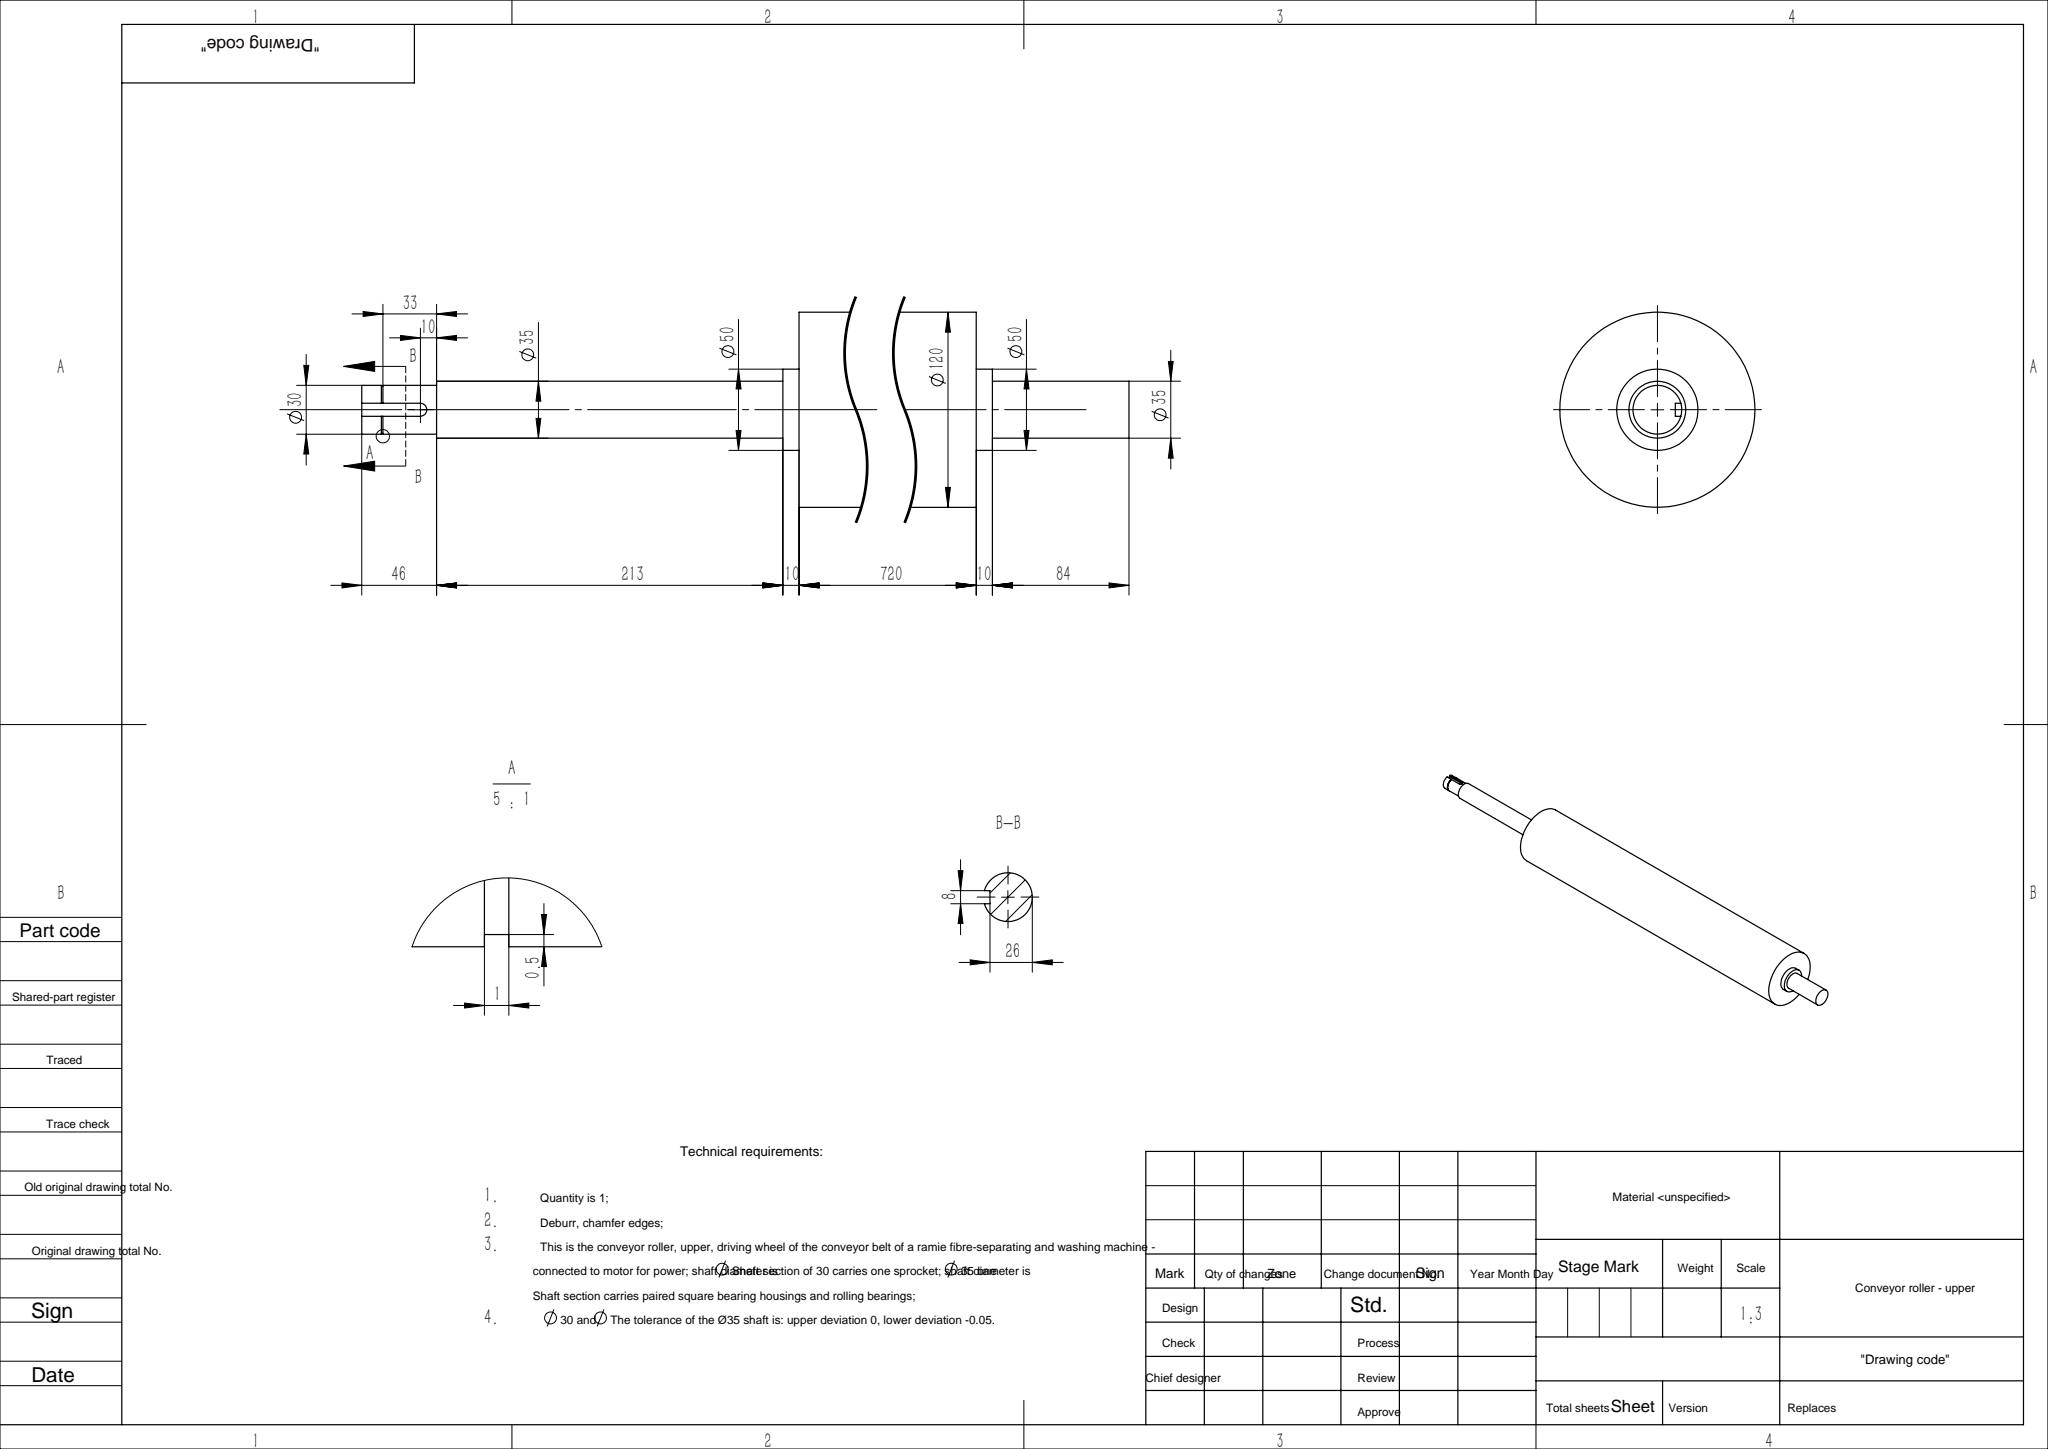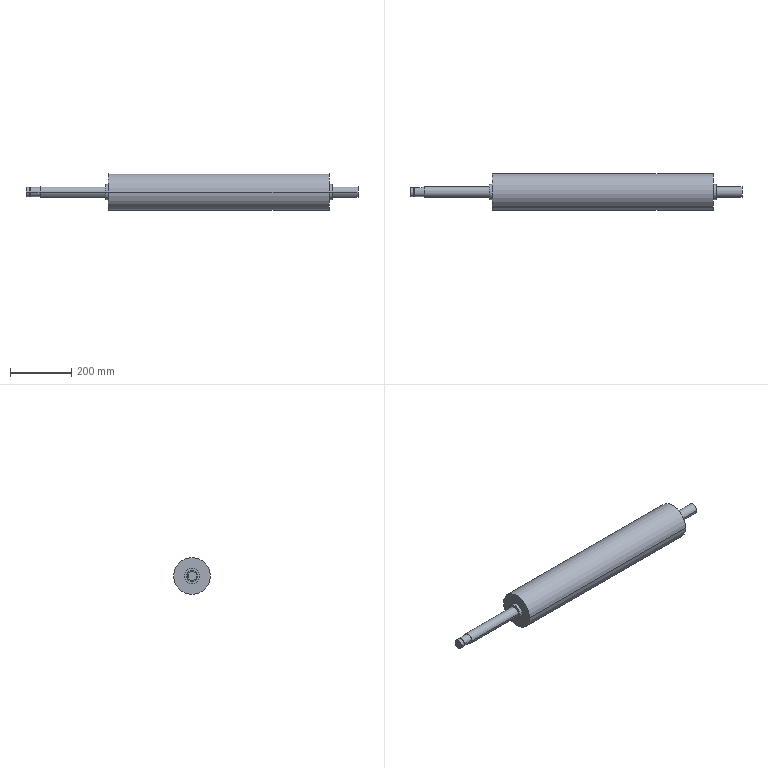Part | SolidWorks | features ICE 2, Revolution 1 | 1 solid | 29 faces | box 1083 x 120 x 120 mm | volume 8499267 mm3 | cylinder 17 | plane 12 | commonest cylinder face diameters 30 x4 35 x4 50 x4 28.6 x2 120 x2 8 x1
STEP:
#1=CARTESIAN_POINT('',(-614.9,13.729,-4.));
#2=VERTEX_POINT('',#1);
#3=CARTESIAN_POINT('',(-614.9,-14.3,0.));
#4=VERTEX_POINT('',#3);
#5=CARTESIAN_POINT('',(-614.9,0.,0.));
#6=DIRECTION('',(-1.,0.,0.));
#7=DIRECTION('',(0.,-1.,0.));
#8=AXIS2_PLACEMENT_3D('',#5,#6,#7);
#9=CIRCLE('',#8,14.3);
#10=EDGE_CURVE('',#2,#4,#9,.T.);
#11=ORIENTED_EDGE('',*,*,#10,.T.);
#12=CARTESIAN_POINT('',(-616.2,-14.3,0.));
#13=VERTEX_POINT('',#12);
#14=CARTESIAN_POINT('',(-614.9,-14.3,0.));
#15=DIRECTION('',(-1.,0.,0.));
#16=VECTOR('',#15,1000.);
#17=LINE('',#14,#16);
#18=EDGE_CURVE('',#4,#13,#17,.T.);
#19=ORIENTED_EDGE('',*,*,#18,.T.);
#20=CARTESIAN_POINT('',(-616.2,13.729,-4.));
#21=VERTEX_POINT('',#20);
#22=CARTESIAN_POINT('',(-616.2,0.,0.));
#23=DIRECTION('',(-1.,0.,0.));
#24=DIRECTION('',(0.,-1.,0.));
#25=AXIS2_PLACEMENT_3D('',#22,#23,#24);
#26=CIRCLE('',#25,14.3);
#27=EDGE_CURVE('',#21,#13,#26,.T.);
#28=ORIENTED_EDGE('',*,*,#27,.F.);
#29=CARTESIAN_POINT('',(-614.9,13.729,-4.));
#30=DIRECTION('',(1.,0.,0.));
#31=VECTOR('',#30,1000.);
#32=LINE('',#29,#31);
#33=EDGE_CURVE('',#21,#2,#32,.T.);
#34=ORIENTED_EDGE('',*,*,#33,.T.);
#35=EDGE_LOOP('',(#11,#19,#28,#34));
#36=FACE_OUTER_BOUND('',#35,.T.);
#37=CARTESIAN_POINT('',(-614.9,0.,0.));
#38=DIRECTION('',(-1.,0.,0.));
#39=DIRECTION('',(0.,-1.,0.));
#40=AXIS2_PLACEMENT_3D('',#37,#38,#39);
#41=CYLINDRICAL_SURFACE('',#40,14.3);
#42=ADVANCED_FACE('',(#36),#41,.T.);
#43=CARTESIAN_POINT('',(-616.2,14.457,-4.));
#44=VERTEX_POINT('',#43);
#45=CARTESIAN_POINT('',(-616.2,-15.,0.));
#46=VERTEX_POINT('',#45);
#47=CARTESIAN_POINT('',(-616.2,0.,0.));
#48=DIRECTION('',(-1.,0.,0.));
#49=DIRECTION('',(0.,-1.,0.));
#50=AXIS2_PLACEMENT_3D('',#47,#48,#49);
#51=CIRCLE('',#50,15.);
#52=EDGE_CURVE('',#44,#46,#51,.T.);
#53=ORIENTED_EDGE('',*,*,#52,.T.);
#54=CARTESIAN_POINT('',(-629.,-15.,0.));
#55=VERTEX_POINT('',#54);
#56=CARTESIAN_POINT('',(-629.,-15.,0.));
#57=DIRECTION('',(-1.,0.,0.));
#58=VECTOR('',#57,1000.);
#59=LINE('',#56,#58);
#60=EDGE_CURVE('',#46,#55,#59,.T.);
#61=ORIENTED_EDGE('',*,*,#60,.T.);
#62=CARTESIAN_POINT('',(-629.,14.457,-4.));
#63=VERTEX_POINT('',#62);
#64=CARTESIAN_POINT('',(-629.,0.,0.));
#65=DIRECTION('',(-1.,0.,0.));
#66=DIRECTION('',(0.,-1.,0.));
#67=AXIS2_PLACEMENT_3D('',#64,#65,#66);
#68=CIRCLE('',#67,15.);
#69=EDGE_CURVE('',#63,#55,#68,.T.);
#70=ORIENTED_EDGE('',*,*,#69,.F.);
#71=CARTESIAN_POINT('',(-629.,14.457,-4.));
#72=DIRECTION('',(1.,0.,0.));
#73=VECTOR('',#72,1000.);
#74=LINE('',#71,#73);
#75=EDGE_CURVE('',#63,#44,#74,.T.);
#76=ORIENTED_EDGE('',*,*,#75,.T.);
#77=EDGE_LOOP('',(#53,#61,#70,#76));
#78=FACE_OUTER_BOUND('',#77,.T.);
#79=CARTESIAN_POINT('',(-629.,0.,0.));
#80=DIRECTION('',(-1.,0.,0.));
#81=DIRECTION('',(0.,-1.,0.));
#82=AXIS2_PLACEMENT_3D('',#79,#80,#81);
#83=CYLINDRICAL_SURFACE('',#82,15.);
#84=ADVANCED_FACE('',(#78),#83,.T.);
#85=CARTESIAN_POINT('',(454.,-17.5,0.));
#86=VERTEX_POINT('',#85);
#87=CARTESIAN_POINT('',(454.,17.5,0.));
#88=VERTEX_POINT('',#87);
#89=CARTESIAN_POINT('',(454.,0.,0.));
#90=DIRECTION('',(-1.,0.,0.));
#91=DIRECTION('',(0.,-1.,0.));
#92=AXIS2_PLACEMENT_3D('',#89,#90,#91);
#93=CIRCLE('',#92,17.5);
#94=EDGE_CURVE('',#86,#88,#93,.T.);
#95=ORIENTED_EDGE('',*,*,#94,.T.);
#96=CARTESIAN_POINT('',(370.,17.5,0.));
#97=VERTEX_POINT('',#96);
#98=CARTESIAN_POINT('',(-629.,17.5,0.));
#99=DIRECTION('',(-1.,0.,0.));
#100=VECTOR('',#99,1000.);
#101=LINE('',#98,#100);
#102=EDGE_CURVE('',#88,#97,#101,.T.);
#103=ORIENTED_EDGE('',*,*,#102,.T.);
#104=CARTESIAN_POINT('',(370.,-17.5,0.));
#105=VERTEX_POINT('',#104);
#106=CARTESIAN_POINT('',(370.,0.,0.));
#107=DIRECTION('',(-1.,0.,0.));
#108=DIRECTION('',(0.,-1.,0.));
#109=AXIS2_PLACEMENT_3D('',#106,#107,#108);
#110=CIRCLE('',#109,17.5);
#111=EDGE_CURVE('',#105,#97,#110,.T.);
#112=ORIENTED_EDGE('',*,*,#111,.F.);
#113=CARTESIAN_POINT('',(-629.,-17.5,0.));
#114=DIRECTION('',(-1.,0.,0.));
#115=VECTOR('',#114,1000.);
#116=LINE('',#113,#115);
#117=EDGE_CURVE('',#86,#105,#116,.T.);
#118=ORIENTED_EDGE('',*,*,#117,.F.);
#119=EDGE_LOOP('',(#95,#103,#112,#118));
#120=FACE_OUTER_BOUND('',#119,.T.);
#121=CARTESIAN_POINT('',(-629.,0.,0.));
#122=DIRECTION('',(-1.,0.,0.));
#123=DIRECTION('',(0.,-1.,0.));
#124=AXIS2_PLACEMENT_3D('',#121,#122,#123);
#125=CYLINDRICAL_SURFACE('',#124,17.5);
#126=ADVANCED_FACE('',(#120),#125,.T.);
#127=CARTESIAN_POINT('',(370.,-25.,0.));
#128=VERTEX_POINT('',#127);
#129=CARTESIAN_POINT('',(370.,25.,0.));
#130=VERTEX_POINT('',#129);
#131=CARTESIAN_POINT('',(370.,0.,0.));
#132=DIRECTION('',(-1.,0.,0.));
#133=DIRECTION('',(0.,-1.,0.));
#134=AXIS2_PLACEMENT_3D('',#131,#132,#133);
#135=CIRCLE('',#134,25.);
#136=EDGE_CURVE('',#128,#130,#135,.T.);
#137=ORIENTED_EDGE('',*,*,#136,.T.);
#138=CARTESIAN_POINT('',(360.,25.,0.));
#139=VERTEX_POINT('',#138);
#140=CARTESIAN_POINT('',(-629.,25.,0.));
#141=DIRECTION('',(-1.,0.,0.));
#142=VECTOR('',#141,1000.);
#143=LINE('',#140,#142);
#144=EDGE_CURVE('',#130,#139,#143,.T.);
#145=ORIENTED_EDGE('',*,*,#144,.T.);
#146=CARTESIAN_POINT('',(360.,-25.,0.));
#147=VERTEX_POINT('',#146);
#148=CARTESIAN_POINT('',(360.,0.,0.));
#149=DIRECTION('',(-1.,0.,0.));
#150=DIRECTION('',(0.,-1.,0.));
#151=AXIS2_PLACEMENT_3D('',#148,#149,#150);
#152=CIRCLE('',#151,25.);
#153=EDGE_CURVE('',#147,#139,#152,.T.);
#154=ORIENTED_EDGE('',*,*,#153,.F.);
#155=CARTESIAN_POINT('',(-629.,-25.,0.));
#156=DIRECTION('',(-1.,0.,0.));
#157=VECTOR('',#156,1000.);
#158=LINE('',#155,#157);
#159=EDGE_CURVE('',#128,#147,#158,.T.);
#160=ORIENTED_EDGE('',*,*,#159,.F.);
#161=EDGE_LOOP('',(#137,#145,#154,#160));
#162=FACE_OUTER_BOUND('',#161,.T.);
#163=CARTESIAN_POINT('',(-629.,0.,0.));
#164=DIRECTION('',(-1.,0.,0.));
#165=DIRECTION('',(0.,-1.,0.));
#166=AXIS2_PLACEMENT_3D('',#163,#164,#165);
#167=CYLINDRICAL_SURFACE('',#166,25.);
#168=ADVANCED_FACE('',(#162),#167,.T.);
#169=CARTESIAN_POINT('',(360.,-60.,0.));
#170=VERTEX_POINT('',#169);
#171=CARTESIAN_POINT('',(360.,60.,0.));
#172=VERTEX_POINT('',#171);
#173=CARTESIAN_POINT('',(360.,0.,0.));
#174=DIRECTION('',(-1.,0.,0.));
#175=DIRECTION('',(0.,-1.,0.));
#176=AXIS2_PLACEMENT_3D('',#173,#174,#175);
#177=CIRCLE('',#176,60.);
#178=EDGE_CURVE('',#170,#172,#177,.T.);
#179=ORIENTED_EDGE('',*,*,#178,.T.);
#180=CARTESIAN_POINT('',(-360.,60.,0.));
#181=VERTEX_POINT('',#180);
#182=CARTESIAN_POINT('',(-629.,60.,0.));
#183=DIRECTION('',(-1.,0.,0.));
#184=VECTOR('',#183,1000.);
#185=LINE('',#182,#184);
#186=EDGE_CURVE('',#172,#181,#185,.T.);
#187=ORIENTED_EDGE('',*,*,#186,.T.);
#188=CARTESIAN_POINT('',(-360.,-60.,0.));
#189=VERTEX_POINT('',#188);
#190=CARTESIAN_POINT('',(-360.,0.,0.));
#191=DIRECTION('',(-1.,0.,0.));
#192=DIRECTION('',(0.,-1.,0.));
#193=AXIS2_PLACEMENT_3D('',#190,#191,#192);
#194=CIRCLE('',#193,60.);
#195=EDGE_CURVE('',#189,#181,#194,.T.);
#196=ORIENTED_EDGE('',*,*,#195,.F.);
#197=CARTESIAN_POINT('',(-629.,-60.,0.));
#198=DIRECTION('',(-1.,0.,0.));
#199=VECTOR('',#198,1000.);
#200=LINE('',#197,#199);
#201=EDGE_CURVE('',#170,#189,#200,.T.);
#202=ORIENTED_EDGE('',*,*,#201,.F.);
#203=EDGE_LOOP('',(#179,#187,#196,#202));
#204=FACE_OUTER_BOUND('',#203,.T.);
#205=CARTESIAN_POINT('',(-629.,0.,0.));
#206=DIRECTION('',(-1.,0.,0.));
#207=DIRECTION('',(0.,-1.,0.));
#208=AXIS2_PLACEMENT_3D('',#205,#206,#207);
#209=CYLINDRICAL_SURFACE('',#208,60.);
#210=ADVANCED_FACE('',(#204),#209,.T.);
#211=CARTESIAN_POINT('',(-360.,-25.,0.));
#212=VERTEX_POINT('',#211);
#213=CARTESIAN_POINT('',(-360.,25.,0.));
#214=VERTEX_POINT('',#213);
#215=CARTESIAN_POINT('',(-360.,0.,0.));
#216=DIRECTION('',(-1.,0.,0.));
#217=DIRECTION('',(0.,-1.,0.));
#218=AXIS2_PLACEMENT_3D('',#215,#216,#217);
#219=CIRCLE('',#218,25.);
#220=EDGE_CURVE('',#212,#214,#219,.T.);
#221=ORIENTED_EDGE('',*,*,#220,.T.);
#222=CARTESIAN_POINT('',(-370.,25.,0.));
#223=VERTEX_POINT('',#222);
#224=CARTESIAN_POINT('',(-629.,25.,0.));
#225=DIRECTION('',(-1.,0.,0.));
#226=VECTOR('',#225,1000.);
#227=LINE('',#224,#226);
#228=EDGE_CURVE('',#214,#223,#227,.T.);
#229=ORIENTED_EDGE('',*,*,#228,.T.);
#230=CARTESIAN_POINT('',(-370.,-25.,0.));
#231=VERTEX_POINT('',#230);
#232=CARTESIAN_POINT('',(-370.,0.,0.));
#233=DIRECTION('',(-1.,0.,0.));
#234=DIRECTION('',(0.,-1.,0.));
#235=AXIS2_PLACEMENT_3D('',#232,#233,#234);
#236=CIRCLE('',#235,25.);
#237=EDGE_CURVE('',#231,#223,#236,.T.);
#238=ORIENTED_EDGE('',*,*,#237,.F.);
#239=CARTESIAN_POINT('',(-629.,-25.,0.));
#240=DIRECTION('',(-1.,0.,0.));
#241=VECTOR('',#240,1000.);
#242=LINE('',#239,#241);
#243=EDGE_CURVE('',#212,#231,#242,.T.);
#244=ORIENTED_EDGE('',*,*,#243,.F.);
#245=EDGE_LOOP('',(#221,#229,#238,#244));
#246=FACE_OUTER_BOUND('',#245,.T.);
#247=CARTESIAN_POINT('',(-629.,0.,0.));
#248=DIRECTION('',(-1.,0.,0.));
#249=DIRECTION('',(0.,-1.,0.));
#250=AXIS2_PLACEMENT_3D('',#247,#248,#249);
#251=CYLINDRICAL_SURFACE('',#250,25.);
#252=ADVANCED_FACE('',(#246),#251,.T.);
#253=CARTESIAN_POINT('',(-370.,-17.5,0.));
#254=VERTEX_POINT('',#253);
#255=CARTESIAN_POINT('',(-370.,17.5,0.));
#256=VERTEX_POINT('',#255);
#257=CARTESIAN_POINT('',(-370.,0.,0.));
#258=DIRECTION('',(-1.,0.,0.));
#259=DIRECTION('',(0.,-1.,0.));
#260=AXIS2_PLACEMENT_3D('',#257,#258,#259);
#261=CIRCLE('',#260,17.5);
#262=EDGE_CURVE('',#254,#256,#261,.T.);
#263=ORIENTED_EDGE('',*,*,#262,.T.);
#264=CARTESIAN_POINT('',(-583.,17.5,0.));
#265=VERTEX_POINT('',#264);
#266=CARTESIAN_POINT('',(-629.,17.5,0.));
#267=DIRECTION('',(-1.,0.,0.));
#268=VECTOR('',#267,1000.);
#269=LINE('',#266,#268);
#270=EDGE_CURVE('',#256,#265,#269,.T.);
#271=ORIENTED_EDGE('',*,*,#270,.T.);
#272=CARTESIAN_POINT('',(-583.,-17.5,0.));
#273=VERTEX_POINT('',#272);
#274=CARTESIAN_POINT('',(-583.,0.,0.));
#275=DIRECTION('',(-1.,0.,0.));
#276=DIRECTION('',(0.,-1.,0.));
#277=AXIS2_PLACEMENT_3D('',#274,#275,#276);
#278=CIRCLE('',#277,17.5);
#279=EDGE_CURVE('',#273,#265,#278,.T.);
#280=ORIENTED_EDGE('',*,*,#279,.F.);
#281=CARTESIAN_POINT('',(-629.,-17.5,0.));
#282=DIRECTION('',(-1.,0.,0.));
#283=VECTOR('',#282,1000.);
#284=LINE('',#281,#283);
#285=EDGE_CURVE('',#254,#273,#284,.T.);
#286=ORIENTED_EDGE('',*,*,#285,.F.);
#287=EDGE_LOOP('',(#263,#271,#280,#286));
#288=FACE_OUTER_BOUND('',#287,.T.);
#289=CARTESIAN_POINT('',(-629.,0.,0.));
#290=DIRECTION('',(-1.,0.,0.));
#291=DIRECTION('',(0.,-1.,0.));
#292=AXIS2_PLACEMENT_3D('',#289,#290,#291);
#293=CYLINDRICAL_SURFACE('',#292,17.5);
#294=ADVANCED_FACE('',(#288),#293,.T.);
#295=CARTESIAN_POINT('',(-583.,-15.,0.));
#296=VERTEX_POINT('',#295);
#297=CARTESIAN_POINT('',(-583.,15.,0.));
#298=VERTEX_POINT('',#297);
#299=CARTESIAN_POINT('',(-583.,0.,0.));
#300=DIRECTION('',(-1.,0.,0.));
#301=DIRECTION('',(0.,-1.,0.));
#302=AXIS2_PLACEMENT_3D('',#299,#300,#301);
#303=CIRCLE('',#302,15.);
#304=EDGE_CURVE('',#296,#298,#303,.T.);
#305=ORIENTED_EDGE('',*,*,#304,.T.);
#306=CARTESIAN_POINT('',(-589.,15.,0.));
#307=VERTEX_POINT('',#306);
#308=CARTESIAN_POINT('',(-629.,15.,0.));
#309=DIRECTION('',(-1.,0.,0.));
#310=VECTOR('',#309,1000.);
#311=LINE('',#308,#310);
#312=EDGE_CURVE('',#298,#307,#311,.T.);
#313=ORIENTED_EDGE('',*,*,#312,.T.);
#314=CARTESIAN_POINT('',(-593.,14.457,4.));
#315=VERTEX_POINT('',#314);
#316=CARTESIAN_POINT('',(-589.,15.,0.));
#317=CARTESIAN_POINT('',(-589.,15.,0.262));
#318=CARTESIAN_POINT('',(-589.026,14.993,0.5282));
#319=CARTESIAN_POINT('',(-589.129,14.966,1.042));
#320=CARTESIAN_POINT('',(-589.205,14.946,1.292));
#321=CARTESIAN_POINT('',(-589.508,14.871,2.02));
#322=CARTESIAN_POINT('',(-589.802,14.802,2.459));
#323=CARTESIAN_POINT('',(-590.357,14.695,3.014));
#324=CARTESIAN_POINT('',(-590.557,14.66,3.178));
#325=CARTESIAN_POINT('',(-590.989,14.594,3.467));
#326=CARTESIAN_POINT('',(-591.223,14.564,3.593));
#327=CARTESIAN_POINT('',(-591.705,14.513,3.794));
#328=CARTESIAN_POINT('',(-591.954,14.492,3.87));
#329=CARTESIAN_POINT('',(-592.469,14.464,3.973));
#330=CARTESIAN_POINT('',(-592.735,14.457,4.));
#331=CARTESIAN_POINT('',(-593.,14.457,4.));
#332=B_SPLINE_CURVE_WITH_KNOTS('',3,(#316,#317,#318,#319,#320,#321,#322,#323,#324,#325,#326,#327,#328,#329,#330,#331),.UNSPECIFIED.,.F.,.F.,(4,2,2,2,2,2,2,4),(0.006283,0.007068,0.007852,0.009421,0.01021,0.01099,0.01177,0.01256),.UNSPECIFIED.);
#333=EDGE_CURVE('',#307,#315,#332,.T.);
#334=ORIENTED_EDGE('',*,*,#333,.T.);
#335=CARTESIAN_POINT('',(-614.9,14.457,4.));
#336=VERTEX_POINT('',#335);
#337=CARTESIAN_POINT('',(-629.,14.457,4.));
#338=DIRECTION('',(-1.,0.,0.));
#339=VECTOR('',#338,1000.);
#340=LINE('',#337,#339);
#341=EDGE_CURVE('',#315,#336,#340,.T.);
#342=ORIENTED_EDGE('',*,*,#341,.T.);
#343=CARTESIAN_POINT('',(-614.9,-15.,0.));
#344=VERTEX_POINT('',#343);
#345=CARTESIAN_POINT('',(-614.9,0.,0.));
#346=DIRECTION('',(-1.,0.,0.));
#347=DIRECTION('',(0.,-1.,0.));
#348=AXIS2_PLACEMENT_3D('',#345,#346,#347);
#349=CIRCLE('',#348,15.);
#350=EDGE_CURVE('',#344,#336,#349,.T.);
#351=ORIENTED_EDGE('',*,*,#350,.F.);
#352=CARTESIAN_POINT('',(-629.,-15.,0.));
#353=DIRECTION('',(-1.,0.,0.));
#354=VECTOR('',#353,1000.);
#355=LINE('',#352,#354);
#356=EDGE_CURVE('',#296,#344,#355,.T.);
#357=ORIENTED_EDGE('',*,*,#356,.F.);
#358=EDGE_LOOP('',(#305,#313,#334,#342,#351,#357));
#359=FACE_OUTER_BOUND('',#358,.T.);
#360=CARTESIAN_POINT('',(-629.,0.,0.));
#361=DIRECTION('',(-1.,0.,0.));
#362=DIRECTION('',(0.,-1.,0.));
#363=AXIS2_PLACEMENT_3D('',#360,#361,#362);
#364=CYLINDRICAL_SURFACE('',#363,15.);
#365=ADVANCED_FACE('',(#359),#364,.T.);
#366=ORIENTED_EDGE('',*,*,#312,.F.);
#367=CARTESIAN_POINT('',(-583.,0.,0.));
#368=DIRECTION('',(-1.,0.,0.));
#369=DIRECTION('',(0.,-1.,0.));
#370=AXIS2_PLACEMENT_3D('',#367,#368,#369);
#371=CIRCLE('',#370,15.);
#372=EDGE_CURVE('',#298,#296,#371,.T.);
#373=ORIENTED_EDGE('',*,*,#372,.T.);
#374=ORIENTED_EDGE('',*,*,#356,.T.);
#375=CARTESIAN_POINT('',(-614.9,14.457,-4.));
#376=VERTEX_POINT('',#375);
#377=CARTESIAN_POINT('',(-614.9,0.,0.));
#378=DIRECTION('',(-1.,0.,0.));
#379=DIRECTION('',(0.,-1.,0.));
#380=AXIS2_PLACEMENT_3D('',#377,#378,#379);
#381=CIRCLE('',#380,15.);
#382=EDGE_CURVE('',#376,#344,#381,.T.);
#383=ORIENTED_EDGE('',*,*,#382,.F.);
#384=CARTESIAN_POINT('',(-593.,14.457,-4.));
#385=VERTEX_POINT('',#384);
#386=CARTESIAN_POINT('',(-629.,14.457,-4.));
#387=DIRECTION('',(1.,0.,0.));
#388=VECTOR('',#387,1000.);
#389=LINE('',#386,#388);
#390=EDGE_CURVE('',#376,#385,#389,.T.);
#391=ORIENTED_EDGE('',*,*,#390,.T.);
#392=CARTESIAN_POINT('',(-593.,14.457,-4.));
#393=CARTESIAN_POINT('',(-592.734,14.457,-4.));
#394=CARTESIAN_POINT('',(-592.473,14.464,-3.974));
#395=CARTESIAN_POINT('',(-591.96,14.492,-3.871));
#396=CARTESIAN_POINT('',(-591.706,14.513,-3.794));
#397=CARTESIAN_POINT('',(-591.222,14.564,-3.593));
#398=CARTESIAN_POINT('',(-590.992,14.594,-3.47));
#399=CARTESIAN_POINT('',(-590.558,14.66,-3.179));
#400=CARTESIAN_POINT('',(-590.354,14.696,-3.011));
#401=CARTESIAN_POINT('',(-589.987,14.766,-2.644));
#402=CARTESIAN_POINT('',(-589.822,14.801,-2.443));
#403=CARTESIAN_POINT('',(-589.529,14.867,-2.006));
#404=CARTESIAN_POINT('',(-589.406,14.897,-1.775));
#405=CARTESIAN_POINT('',(-589.206,14.946,-1.293));
#406=CARTESIAN_POINT('',(-589.129,14.966,-1.04));
#407=CARTESIAN_POINT('',(-589.026,14.993,-0.5228));
#408=CARTESIAN_POINT('',(-589.,15.,-0.2623));
#409=CARTESIAN_POINT('',(-589.,15.,0.));
#410=B_SPLINE_CURVE_WITH_KNOTS('',3,(#392,#393,#394,#395,#396,#397,#398,#399,#400,#401,#402,#403,#404,#405,#406,#407,#408,#409),.UNSPECIFIED.,.F.,.F.,(4,2,2,2,2,2,2,2,4),(0.,0.0007854,0.001571,0.002356,0.003142,0.003927,0.004712,0.005498,0.006283),.UNSPECIFIED.);
#411=EDGE_CURVE('',#385,#307,#410,.T.);
#412=ORIENTED_EDGE('',*,*,#411,.T.);
#413=EDGE_LOOP('',(#366,#373,#374,#383,#391,#412));
#414=FACE_OUTER_BOUND('',#413,.T.);
#415=CARTESIAN_POINT('',(-629.,0.,0.));
#416=DIRECTION('',(-1.,0.,0.));
#417=DIRECTION('',(0.,-1.,0.));
#418=AXIS2_PLACEMENT_3D('',#415,#416,#417);
#419=CYLINDRICAL_SURFACE('',#418,15.);
#420=ADVANCED_FACE('',(#414),#419,.T.);
#421=CARTESIAN_POINT('',(-614.9,11.,-4.));
#422=DIRECTION('',(0.,1.,0.));
#423=VECTOR('',#422,1000.);
#424=LINE('',#421,#423);
#425=EDGE_CURVE('',#2,#376,#424,.T.);
#426=ORIENTED_EDGE('',*,*,#425,.F.);
#427=ORIENTED_EDGE('',*,*,#33,.F.);
#428=CARTESIAN_POINT('',(-616.2,11.,-4.));
#429=DIRECTION('',(0.,1.,0.));
#430=VECTOR('',#429,1000.);
#431=LINE('',#428,#430);
#432=EDGE_CURVE('',#21,#44,#431,.T.);
#433=ORIENTED_EDGE('',*,*,#432,.T.);
#434=ORIENTED_EDGE('',*,*,#75,.F.);
#435=CARTESIAN_POINT('',(-629.,11.,-4.));
#436=VERTEX_POINT('',#435);
#437=CARTESIAN_POINT('',(-629.,11.,-4.));
#438=DIRECTION('',(0.,1.,0.));
#439=VECTOR('',#438,1000.);
#440=LINE('',#437,#439);
#441=EDGE_CURVE('',#436,#63,#440,.T.);
#442=ORIENTED_EDGE('',*,*,#441,.F.);
#443=CARTESIAN_POINT('',(-593.,11.,-4.));
#444=VERTEX_POINT('',#443);
#445=CARTESIAN_POINT('',(-629.,11.,-4.));
#446=DIRECTION('',(-1.,0.,0.));
#447=VECTOR('',#446,1000.);
#448=LINE('',#445,#447);
#449=EDGE_CURVE('',#444,#436,#448,.T.);
#450=ORIENTED_EDGE('',*,*,#449,.F.);
#451=CARTESIAN_POINT('',(-593.,11.,-4.));
#452=DIRECTION('',(0.,1.,0.));
#453=VECTOR('',#452,1000.);
#454=LINE('',#451,#453);
#455=EDGE_CURVE('',#444,#385,#454,.T.);
#456=ORIENTED_EDGE('',*,*,#455,.T.);
#457=ORIENTED_EDGE('',*,*,#390,.F.);
#458=EDGE_LOOP('',(#426,#427,#433,#434,#442,#450,#456,#457));
#459=FACE_OUTER_BOUND('',#458,.T.);
#460=CARTESIAN_POINT('',(-629.,11.,-4.));
#461=DIRECTION('',(0.,0.,-1.));
#462=DIRECTION('',(-1.,0.,0.));
#463=AXIS2_PLACEMENT_3D('',#460,#461,#462);
#464=PLANE('',#463);
#465=ADVANCED_FACE('',(#459),#464,.F.);
#466=CARTESIAN_POINT('',(-614.9,13.729,4.));
#467=VERTEX_POINT('',#466);
#468=CARTESIAN_POINT('',(-614.9,11.,4.));
#469=DIRECTION('',(0.,-1.,0.));
#470=VECTOR('',#469,1000.);
#471=LINE('',#468,#470);
#472=EDGE_CURVE('',#336,#467,#471,.T.);
#473=ORIENTED_EDGE('',*,*,#472,.F.);
#474=ORIENTED_EDGE('',*,*,#341,.F.);
#475=CARTESIAN_POINT('',(-593.,11.,4.));
#476=VERTEX_POINT('',#475);
#477=CARTESIAN_POINT('',(-593.,11.,4.));
#478=DIRECTION('',(0.,1.,0.));
#479=VECTOR('',#478,1000.);
#480=LINE('',#477,#479);
#481=EDGE_CURVE('',#476,#315,#480,.T.);
#482=ORIENTED_EDGE('',*,*,#481,.F.);
#483=CARTESIAN_POINT('',(-629.,11.,4.));
#484=VERTEX_POINT('',#483);
#485=CARTESIAN_POINT('',(-629.,11.,4.));
#486=DIRECTION('',(1.,0.,0.));
#487=VECTOR('',#486,1000.);
#488=LINE('',#485,#487);
#489=EDGE_CURVE('',#484,#476,#488,.T.);
#490=ORIENTED_EDGE('',*,*,#489,.F.);
#491=CARTESIAN_POINT('',(-629.,14.457,4.));
#492=VERTEX_POINT('',#491);
#493=CARTESIAN_POINT('',(-629.,11.,4.));
#494=DIRECTION('',(0.,1.,0.));
#495=VECTOR('',#494,1000.);
#496=LINE('',#493,#495);
#497=EDGE_CURVE('',#484,#492,#496,.T.);
#498=ORIENTED_EDGE('',*,*,#497,.T.);
#499=CARTESIAN_POINT('',(-616.2,14.457,4.));
#500=VERTEX_POINT('',#499);
#501=CARTESIAN_POINT('',(-629.,14.457,4.));
#502=DIRECTION('',(-1.,0.,0.));
#503=VECTOR('',#502,1000.);
#504=LINE('',#501,#503);
#505=EDGE_CURVE('',#500,#492,#504,.T.);
#506=ORIENTED_EDGE('',*,*,#505,.F.);
#507=CARTESIAN_POINT('',(-616.2,13.729,4.));
#508=VERTEX_POINT('',#507);
#509=CARTESIAN_POINT('',(-616.2,11.,4.));
#510=DIRECTION('',(0.,-1.,0.));
#511=VECTOR('',#510,1000.);
#512=LINE('',#509,#511);
#513=EDGE_CURVE('',#500,#508,#512,.T.);
#514=ORIENTED_EDGE('',*,*,#513,.T.);
#515=CARTESIAN_POINT('',(-614.9,13.729,4.));
#516=DIRECTION('',(-1.,0.,0.));
#517=VECTOR('',#516,1000.);
#518=LINE('',#515,#517);
#519=EDGE_CURVE('',#467,#508,#518,.T.);
#520=ORIENTED_EDGE('',*,*,#519,.F.);
#521=EDGE_LOOP('',(#473,#474,#482,#490,#498,#506,#514,#520));
#522=FACE_OUTER_BOUND('',#521,.T.);
#523=CARTESIAN_POINT('',(-629.,11.,4.));
#524=DIRECTION('',(0.,0.,1.));
#525=DIRECTION('',(1.,0.,0.));
#526=AXIS2_PLACEMENT_3D('',#523,#524,#525);
#527=PLANE('',#526);
#528=ADVANCED_FACE('',(#522),#527,.F.);
#529=ORIENTED_EDGE('',*,*,#304,.F.);
#530=ORIENTED_EDGE('',*,*,#372,.F.);
#531=EDGE_LOOP('',(#529,#530));
#532=FACE_BOUND('',#531,.T.);
#533=ORIENTED_EDGE('',*,*,#279,.T.);
#534=CARTESIAN_POINT('',(-583.,0.,0.));
#535=DIRECTION('',(-1.,0.,0.));
#536=DIRECTION('',(0.,-1.,0.));
#537=AXIS2_PLACEMENT_3D('',#534,#535,#536);
#538=CIRCLE('',#537,17.5);
#539=EDGE_CURVE('',#265,#273,#538,.T.);
#540=ORIENTED_EDGE('',*,*,#539,.T.);
#541=EDGE_LOOP('',(#533,#540));
#542=FACE_OUTER_BOUND('',#541,.T.);
#543=CARTESIAN_POINT('',(-583.,17.5,0.));
#544=DIRECTION('',(1.,0.,0.));
#545=DIRECTION('',(0.,1.,0.));
#546=AXIS2_PLACEMENT_3D('',#543,#544,#545);
#547=PLANE('',#546);
#548=ADVANCED_FACE('',(#532,#542),#547,.F.);
#549=ORIENTED_EDGE('',*,*,#270,.F.);
#550=CARTESIAN_POINT('',(-370.,0.,0.));
#551=DIRECTION('',(-1.,0.,0.));
#552=DIRECTION('',(0.,-1.,0.));
#553=AXIS2_PLACEMENT_3D('',#550,#551,#552);
#554=CIRCLE('',#553,17.5);
#555=EDGE_CURVE('',#256,#254,#554,.T.);
#556=ORIENTED_EDGE('',*,*,#555,.T.);
#557=ORIENTED_EDGE('',*,*,#285,.T.);
#558=ORIENTED_EDGE('',*,*,#539,.F.);
#559=EDGE_LOOP('',(#549,#556,#557,#558));
#560=FACE_OUTER_BOUND('',#559,.T.);
#561=CARTESIAN_POINT('',(-629.,0.,0.));
#562=DIRECTION('',(-1.,0.,0.));
#563=DIRECTION('',(0.,-1.,0.));
#564=AXIS2_PLACEMENT_3D('',#561,#562,#563);
#565=CYLINDRICAL_SURFACE('',#564,17.5);
#566=ADVANCED_FACE('',(#560),#565,.T.);
#567=ORIENTED_EDGE('',*,*,#262,.F.);
#568=ORIENTED_EDGE('',*,*,#555,.F.);
#569=EDGE_LOOP('',(#567,#568));
#570=FACE_BOUND('',#569,.T.);
#571=ORIENTED_EDGE('',*,*,#237,.T.);
#572=CARTESIAN_POINT('',(-370.,0.,0.));
#573=DIRECTION('',(-1.,0.,0.));
#574=DIRECTION('',(0.,-1.,0.));
#575=AXIS2_PLACEMENT_3D('',#572,#573,#574);
#576=CIRCLE('',#575,25.);
#577=EDGE_CURVE('',#223,#231,#576,.T.);
#578=ORIENTED_EDGE('',*,*,#577,.T.);
#579=EDGE_LOOP('',(#571,#578));
#580=FACE_OUTER_BOUND('',#579,.T.);
#581=CARTESIAN_POINT('',(-370.,25.,0.));
#582=DIRECTION('',(1.,0.,0.));
#583=DIRECTION('',(0.,1.,0.));
#584=AXIS2_PLACEMENT_3D('',#581,#582,#583);
#585=PLANE('',#584);
#586=ADVANCED_FACE('',(#570,#580),#585,.F.);
#587=ORIENTED_EDGE('',*,*,#228,.F.);
#588=CARTESIAN_POINT('',(-360.,0.,0.));
#589=DIRECTION('',(-1.,0.,0.));
#590=DIRECTION('',(0.,-1.,0.));
#591=AXIS2_PLACEMENT_3D('',#588,#589,#590);
#592=CIRCLE('',#591,25.);
#593=EDGE_CURVE('',#214,#212,#592,.T.);
#594=ORIENTED_EDGE('',*,*,#593,.T.);
#595=ORIENTED_EDGE('',*,*,#243,.T.);
#596=ORIENTED_EDGE('',*,*,#577,.F.);
#597=EDGE_LOOP('',(#587,#594,#595,#596));
#598=FACE_OUTER_BOUND('',#597,.T.);
#599=CARTESIAN_POINT('',(-629.,0.,0.));
#600=DIRECTION('',(-1.,0.,0.));
#601=DIRECTION('',(0.,-1.,0.));
#602=AXIS2_PLACEMENT_3D('',#599,#600,#601);
#603=CYLINDRICAL_SURFACE('',#602,25.);
#604=ADVANCED_FACE('',(#598),#603,.T.);
#605=ORIENTED_EDGE('',*,*,#220,.F.);
#606=ORIENTED_EDGE('',*,*,#593,.F.);
#607=EDGE_LOOP('',(#605,#606));
#608=FACE_BOUND('',#607,.T.);
#609=ORIENTED_EDGE('',*,*,#195,.T.);
#610=CARTESIAN_POINT('',(-360.,0.,0.));
#611=DIRECTION('',(-1.,0.,0.));
#612=DIRECTION('',(0.,-1.,0.));
#613=AXIS2_PLACEMENT_3D('',#610,#611,#612);
#614=CIRCLE('',#613,60.);
#615=EDGE_CURVE('',#181,#189,#614,.T.);
#616=ORIENTED_EDGE('',*,*,#615,.T.);
#617=EDGE_LOOP('',(#609,#616));
#618=FACE_OUTER_BOUND('',#617,.T.);
#619=CARTESIAN_POINT('',(-360.,60.,0.));
#620=DIRECTION('',(1.,0.,0.));
#621=DIRECTION('',(0.,1.,0.));
#622=AXIS2_PLACEMENT_3D('',#619,#620,#621);
#623=PLANE('',#622);
#624=ADVANCED_FACE('',(#608,#618),#623,.F.);
#625=ORIENTED_EDGE('',*,*,#186,.F.);
#626=CARTESIAN_POINT('',(360.,0.,0.));
#627=DIRECTION('',(-1.,0.,0.));
#628=DIRECTION('',(0.,-1.,0.));
#629=AXIS2_PLACEMENT_3D('',#626,#627,#628);
#630=CIRCLE('',#629,60.);
#631=EDGE_CURVE('',#172,#170,#630,.T.);
#632=ORIENTED_EDGE('',*,*,#631,.T.);
#633=ORIENTED_EDGE('',*,*,#201,.T.);
#634=ORIENTED_EDGE('',*,*,#615,.F.);
#635=EDGE_LOOP('',(#625,#632,#633,#634));
#636=FACE_OUTER_BOUND('',#635,.T.);
#637=CARTESIAN_POINT('',(-629.,0.,0.));
#638=DIRECTION('',(-1.,0.,0.));
#639=DIRECTION('',(0.,-1.,0.));
#640=AXIS2_PLACEMENT_3D('',#637,#638,#639);
#641=CYLINDRICAL_SURFACE('',#640,60.);
#642=ADVANCED_FACE('',(#636),#641,.T.);
#643=ORIENTED_EDGE('',*,*,#178,.F.);
#644=ORIENTED_EDGE('',*,*,#631,.F.);
#645=EDGE_LOOP('',(#643,#644));
#646=FACE_OUTER_BOUND('',#645,.T.);
#647=ORIENTED_EDGE('',*,*,#153,.T.);
#648=CARTESIAN_POINT('',(360.,0.,0.));
#649=DIRECTION('',(-1.,0.,0.));
#650=DIRECTION('',(0.,-1.,0.));
#651=AXIS2_PLACEMENT_3D('',#648,#649,#650);
#652=CIRCLE('',#651,25.);
#653=EDGE_CURVE('',#139,#147,#652,.T.);
#654=ORIENTED_EDGE('',*,*,#653,.T.);
#655=EDGE_LOOP('',(#647,#654));
#656=FACE_BOUND('',#655,.T.);
#657=CARTESIAN_POINT('',(360.,60.,0.));
#658=DIRECTION('',(-1.,0.,0.));
#659=DIRECTION('',(0.,-1.,0.));
#660=AXIS2_PLACEMENT_3D('',#657,#658,#659);
#661=PLANE('',#660);
#662=ADVANCED_FACE('',(#646,#656),#661,.F.);
#663=ORIENTED_EDGE('',*,*,#144,.F.);
#664=CARTESIAN_POINT('',(370.,0.,0.));
#665=DIRECTION('',(-1.,0.,0.));
#666=DIRECTION('',(0.,-1.,0.));
#667=AXIS2_PLACEMENT_3D('',#664,#665,#666);
#668=CIRCLE('',#667,25.);
#669=EDGE_CURVE('',#130,#128,#668,.T.);
#670=ORIENTED_EDGE('',*,*,#669,.T.);
#671=ORIENTED_EDGE('',*,*,#159,.T.);
#672=ORIENTED_EDGE('',*,*,#653,.F.);
#673=EDGE_LOOP('',(#663,#670,#671,#672));
#674=FACE_OUTER_BOUND('',#673,.T.);
#675=CARTESIAN_POINT('',(-629.,0.,0.));
#676=DIRECTION('',(-1.,0.,0.));
#677=DIRECTION('',(0.,-1.,0.));
#678=AXIS2_PLACEMENT_3D('',#675,#676,#677);
#679=CYLINDRICAL_SURFACE('',#678,25.);
#680=ADVANCED_FACE('',(#674),#679,.T.);
#681=ORIENTED_EDGE('',*,*,#136,.F.);
#682=ORIENTED_EDGE('',*,*,#669,.F.);
#683=EDGE_LOOP('',(#681,#682));
#684=FACE_OUTER_BOUND('',#683,.T.);
#685=ORIENTED_EDGE('',*,*,#111,.T.);
#686=CARTESIAN_POINT('',(370.,0.,0.));
#687=DIRECTION('',(-1.,0.,0.));
#688=DIRECTION('',(0.,-1.,0.));
#689=AXIS2_PLACEMENT_3D('',#686,#687,#688);
#690=CIRCLE('',#689,17.5);
#691=EDGE_CURVE('',#97,#105,#690,.T.);
#692=ORIENTED_EDGE('',*,*,#691,.T.);
#693=EDGE_LOOP('',(#685,#692));
#694=FACE_BOUND('',#693,.T.);
#695=CARTESIAN_POINT('',(370.,25.,0.));
#696=DIRECTION('',(-1.,0.,0.));
#697=DIRECTION('',(0.,-1.,0.));
#698=AXIS2_PLACEMENT_3D('',#695,#696,#697);
#699=PLANE('',#698);
#700=ADVANCED_FACE('',(#684,#694),#699,.F.);
#701=ORIENTED_EDGE('',*,*,#102,.F.);
#702=CARTESIAN_POINT('',(454.,0.,0.));
#703=DIRECTION('',(-1.,0.,0.));
#704=DIRECTION('',(0.,-1.,0.));
#705=AXIS2_PLACEMENT_3D('',#702,#703,#704);
#706=CIRCLE('',#705,17.5);
#707=EDGE_CURVE('',#88,#86,#706,.T.);
#708=ORIENTED_EDGE('',*,*,#707,.T.);
#709=ORIENTED_EDGE('',*,*,#117,.T.);
#710=ORIENTED_EDGE('',*,*,#691,.F.);
#711=EDGE_LOOP('',(#701,#708,#709,#710));
#712=FACE_OUTER_BOUND('',#711,.T.);
#713=CARTESIAN_POINT('',(-629.,0.,0.));
#714=DIRECTION('',(-1.,0.,0.));
#715=DIRECTION('',(0.,-1.,0.));
#716=AXIS2_PLACEMENT_3D('',#713,#714,#715);
#717=CYLINDRICAL_SURFACE('',#716,17.5);
#718=ADVANCED_FACE('',(#712),#717,.T.);
#719=ORIENTED_EDGE('',*,*,#94,.F.);
#720=ORIENTED_EDGE('',*,*,#707,.F.);
#721=EDGE_LOOP('',(#719,#720));
#722=FACE_OUTER_BOUND('',#721,.T.);
#723=CARTESIAN_POINT('',(454.,17.5,0.));
#724=DIRECTION('',(-1.,0.,0.));
#725=DIRECTION('',(0.,-1.,0.));
#726=AXIS2_PLACEMENT_3D('',#723,#724,#725);
#727=PLANE('',#726);
#728=ADVANCED_FACE('',(#722),#727,.F.);
#729=CARTESIAN_POINT('',(-629.,11.,-4.));
#730=DIRECTION('',(0.,0.,1.));
#731=VECTOR('',#730,1000.);
#732=LINE('',#729,#731);
#733=EDGE_CURVE('',#436,#484,#732,.T.);
#734=ORIENTED_EDGE('',*,*,#733,.F.);
#735=ORIENTED_EDGE('',*,*,#441,.T.);
#736=ORIENTED_EDGE('',*,*,#69,.T.);
#737=CARTESIAN_POINT('',(-629.,0.,0.));
#738=DIRECTION('',(-1.,0.,0.));
#739=DIRECTION('',(0.,-1.,0.));
#740=AXIS2_PLACEMENT_3D('',#737,#738,#739);
#741=CIRCLE('',#740,15.);
#742=EDGE_CURVE('',#55,#492,#741,.T.);
#743=ORIENTED_EDGE('',*,*,#742,.T.);
#744=ORIENTED_EDGE('',*,*,#497,.F.);
#745=EDGE_LOOP('',(#734,#735,#736,#743,#744));
#746=FACE_OUTER_BOUND('',#745,.T.);
#747=CARTESIAN_POINT('',(-629.,15.,0.));
#748=DIRECTION('',(1.,0.,0.));
#749=DIRECTION('',(0.,1.,0.));
#750=AXIS2_PLACEMENT_3D('',#747,#748,#749);
#751=PLANE('',#750);
#752=ADVANCED_FACE('',(#746),#751,.F.);
#753=ORIENTED_EDGE('',*,*,#60,.F.);
#754=CARTESIAN_POINT('',(-616.2,0.,0.));
#755=DIRECTION('',(-1.,0.,0.));
#756=DIRECTION('',(0.,-1.,0.));
#757=AXIS2_PLACEMENT_3D('',#754,#755,#756);
#758=CIRCLE('',#757,15.);
#759=EDGE_CURVE('',#46,#500,#758,.T.);
#760=ORIENTED_EDGE('',*,*,#759,.T.);
#761=ORIENTED_EDGE('',*,*,#505,.T.);
#762=ORIENTED_EDGE('',*,*,#742,.F.);
#763=EDGE_LOOP('',(#753,#760,#761,#762));
#764=FACE_OUTER_BOUND('',#763,.T.);
#765=CARTESIAN_POINT('',(-629.,0.,0.));
#766=DIRECTION('',(-1.,0.,0.));
#767=DIRECTION('',(0.,-1.,0.));
#768=AXIS2_PLACEMENT_3D('',#765,#766,#767);
#769=CYLINDRICAL_SURFACE('',#768,15.);
#770=ADVANCED_FACE('',(#764),#769,.T.);
#771=ORIENTED_EDGE('',*,*,#455,.F.);
#772=CARTESIAN_POINT('',(-593.,11.,0.));
#773=DIRECTION('',(0.,1.,0.));
#774=DIRECTION('',(-1.,0.,0.));
#775=AXIS2_PLACEMENT_3D('',#772,#773,#774);
#776=CIRCLE('',#775,4.);
#777=EDGE_CURVE('',#476,#444,#776,.T.);
#778=ORIENTED_EDGE('',*,*,#777,.F.);
#779=ORIENTED_EDGE('',*,*,#481,.T.);
#780=ORIENTED_EDGE('',*,*,#333,.F.);
#781=ORIENTED_EDGE('',*,*,#411,.F.);
#782=EDGE_LOOP('',(#771,#778,#779,#780,#781));
#783=FACE_OUTER_BOUND('',#782,.T.);
#784=CARTESIAN_POINT('',(-593.,11.,0.));
#785=DIRECTION('',(0.,1.,0.));
#786=DIRECTION('',(-1.,0.,0.));
#787=AXIS2_PLACEMENT_3D('',#784,#785,#786);
#788=CYLINDRICAL_SURFACE('',#787,4.);
#789=ADVANCED_FACE('',(#783),#788,.F.);
#790=ORIENTED_EDGE('',*,*,#733,.T.);
#791=ORIENTED_EDGE('',*,*,#489,.T.);
#792=ORIENTED_EDGE('',*,*,#777,.T.);
#793=ORIENTED_EDGE('',*,*,#449,.T.);
#794=EDGE_LOOP('',(#790,#791,#792,#793));
#795=FACE_OUTER_BOUND('',#794,.T.);
#796=CARTESIAN_POINT('',(-593.,11.,0.));
#797=DIRECTION('',(0.,1.,0.));
#798=DIRECTION('',(-1.,0.,0.));
#799=AXIS2_PLACEMENT_3D('',#796,#797,#798);
#800=PLANE('',#799);
#801=ADVANCED_FACE('',(#795),#800,.T.);
#802=ORIENTED_EDGE('',*,*,#425,.T.);
#803=ORIENTED_EDGE('',*,*,#382,.T.);
#804=ORIENTED_EDGE('',*,*,#350,.T.);
#805=ORIENTED_EDGE('',*,*,#472,.T.);
#806=CARTESIAN_POINT('',(-614.9,0.,0.));
#807=DIRECTION('',(-1.,0.,0.));
#808=DIRECTION('',(0.,-1.,0.));
#809=AXIS2_PLACEMENT_3D('',#806,#807,#808);
#810=CIRCLE('',#809,14.3);
#811=EDGE_CURVE('',#4,#467,#810,.T.);
#812=ORIENTED_EDGE('',*,*,#811,.F.);
#813=ORIENTED_EDGE('',*,*,#10,.F.);
#814=EDGE_LOOP('',(#802,#803,#804,#805,#812,#813));
#815=FACE_OUTER_BOUND('',#814,.T.);
#816=CARTESIAN_POINT('',(-614.9,0.,0.));
#817=DIRECTION('',(-1.,0.,0.));
#818=DIRECTION('',(0.,-1.,0.));
#819=AXIS2_PLACEMENT_3D('',#816,#817,#818);
#820=PLANE('',#819);
#821=ADVANCED_FACE('',(#815),#820,.T.);
#822=ORIENTED_EDGE('',*,*,#27,.T.);
#823=CARTESIAN_POINT('',(-616.2,0.,0.));
#824=DIRECTION('',(-1.,0.,0.));
#825=DIRECTION('',(0.,-1.,0.));
#826=AXIS2_PLACEMENT_3D('',#823,#824,#825);
#827=CIRCLE('',#826,14.3);
#828=EDGE_CURVE('',#13,#508,#827,.T.);
#829=ORIENTED_EDGE('',*,*,#828,.T.);
#830=ORIENTED_EDGE('',*,*,#513,.F.);
#831=ORIENTED_EDGE('',*,*,#759,.F.);
#832=ORIENTED_EDGE('',*,*,#52,.F.);
#833=ORIENTED_EDGE('',*,*,#432,.F.);
#834=EDGE_LOOP('',(#822,#829,#830,#831,#832,#833));
#835=FACE_OUTER_BOUND('',#834,.T.);
#836=CARTESIAN_POINT('',(-616.2,0.,0.));
#837=DIRECTION('',(-1.,0.,0.));
#838=DIRECTION('',(0.,-1.,0.));
#839=AXIS2_PLACEMENT_3D('',#836,#837,#838);
#840=PLANE('',#839);
#841=ADVANCED_FACE('',(#835),#840,.F.);
#842=ORIENTED_EDGE('',*,*,#18,.F.);
#843=ORIENTED_EDGE('',*,*,#811,.T.);
#844=ORIENTED_EDGE('',*,*,#519,.T.);
#845=ORIENTED_EDGE('',*,*,#828,.F.);
#846=EDGE_LOOP('',(#842,#843,#844,#845));
#847=FACE_OUTER_BOUND('',#846,.T.);
#848=CARTESIAN_POINT('',(-614.9,0.,0.));
#849=DIRECTION('',(-1.,0.,0.));
#850=DIRECTION('',(0.,-1.,0.));
#851=AXIS2_PLACEMENT_3D('',#848,#849,#850);
#852=CYLINDRICAL_SURFACE('',#851,14.3);
#853=ADVANCED_FACE('',(#847),#852,.T.);
#854=CLOSED_SHELL('',(#42,#84,#126,#168,#210,#252,#294,#365,#420,#465,#528,#548,#566,#586,#604,#624,#642,#662,#680,#700,#718,#728,#752,#770,#789,#801,#821,#841,#853));
#855=MANIFOLD_SOLID_BREP('',#854);
#856=CARTESIAN_POINT('',(0.,0.,0.));
#857=DIRECTION('',(0.,0.,1.));
#858=DIRECTION('',(1.,0.,0.));
#859=AXIS2_PLACEMENT_3D('',#856,#857,#858);
#860=(LENGTH_UNIT()NAMED_UNIT(*)SI_UNIT(.MILLI.,.METRE.));
#861=UNCERTAINTY_MEASURE_WITH_UNIT(LENGTH_MEASURE(0.00001),#860,'','');
#862=(NAMED_UNIT(*)PLANE_ANGLE_UNIT()SI_UNIT($,.RADIAN.));
#863=(NAMED_UNIT(*)SI_UNIT($,.STERADIAN.)SOLID_ANGLE_UNIT());
#864=(GEOMETRIC_REPRESENTATION_CONTEXT(3)GLOBAL_UNCERTAINTY_ASSIGNED_CONTEXT((#861))GLOBAL_UNIT_ASSIGNED_CONTEXT((#860,#862,#863))REPRESENTATION_CONTEXT('',''));
#865=ADVANCED_BREP_SHAPE_REPRESENTATION('',(#855,#859),#864);